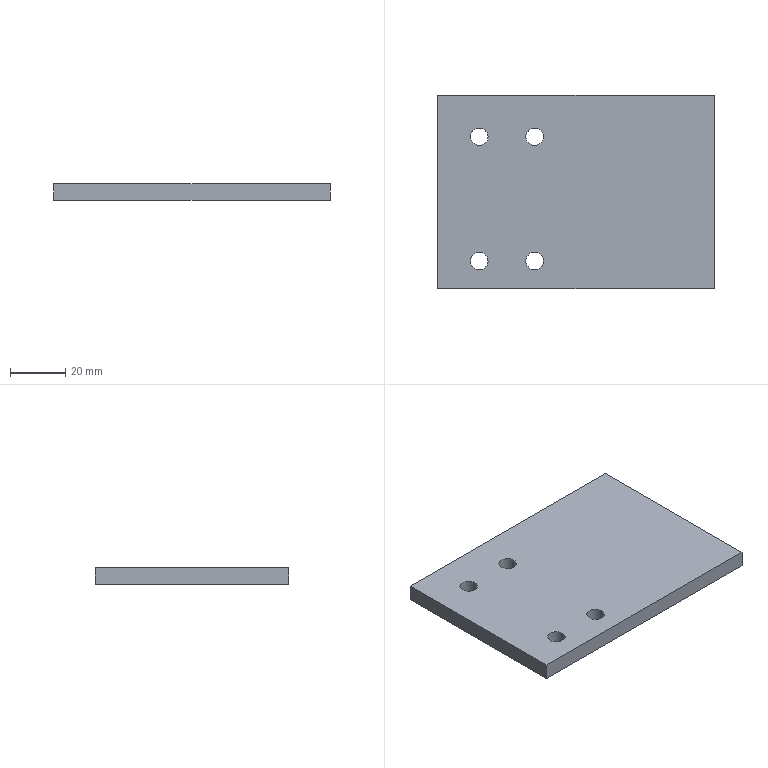Part | SolidWorks | features BaseBody 1 | 1 solid | 14 faces | box 100 x 70 x 6 mm | volume 41252 mm3 | cylinder 8 | plane 6 | commonest cylinder face diameters 6.3 x8
STEP:
#1=CARTESIAN_POINT('',(-18.15,20.,-3.));
#2=VERTEX_POINT('',#1);
#3=CARTESIAN_POINT('',(-11.85,20.,-3.));
#4=VERTEX_POINT('',#3);
#5=CARTESIAN_POINT('',(-15.,20.,-3.));
#6=DIRECTION('',(0.,0.,1.));
#7=DIRECTION('',(1.,0.,0.));
#8=AXIS2_PLACEMENT_3D('',#5,#6,#7);
#9=CIRCLE('',#8,3.15);
#10=EDGE_CURVE('',#2,#4,#9,.T.);
#11=ORIENTED_EDGE('',*,*,#10,.F.);
#12=CARTESIAN_POINT('',(-18.15,20.,3.));
#13=VERTEX_POINT('',#12);
#14=CARTESIAN_POINT('',(-18.15,20.,-15.2));
#15=DIRECTION('',(0.,0.,1.));
#16=VECTOR('',#15,1000.);
#17=LINE('',#14,#16);
#18=EDGE_CURVE('',#2,#13,#17,.T.);
#19=ORIENTED_EDGE('',*,*,#18,.T.);
#20=CARTESIAN_POINT('',(-11.85,20.,3.));
#21=VERTEX_POINT('',#20);
#22=CARTESIAN_POINT('',(-15.,20.,3.));
#23=DIRECTION('',(0.,0.,-1.));
#24=DIRECTION('',(1.,0.,0.));
#25=AXIS2_PLACEMENT_3D('',#22,#23,#24);
#26=CIRCLE('',#25,3.15);
#27=EDGE_CURVE('',#21,#13,#26,.T.);
#28=ORIENTED_EDGE('',*,*,#27,.F.);
#29=CARTESIAN_POINT('',(-11.85,20.,-15.2));
#30=DIRECTION('',(0.,0.,1.));
#31=VECTOR('',#30,1000.);
#32=LINE('',#29,#31);
#33=EDGE_CURVE('',#4,#21,#32,.T.);
#34=ORIENTED_EDGE('',*,*,#33,.F.);
#35=EDGE_LOOP('',(#11,#19,#28,#34));
#36=FACE_OUTER_BOUND('',#35,.T.);
#37=CARTESIAN_POINT('',(-15.,20.,-15.2));
#38=DIRECTION('',(0.,0.,1.));
#39=DIRECTION('',(1.,0.,0.));
#40=AXIS2_PLACEMENT_3D('',#37,#38,#39);
#41=CYLINDRICAL_SURFACE('',#40,3.15);
#42=ADVANCED_FACE('',(#36),#41,.F.);
#43=CARTESIAN_POINT('',(-38.15,20.,-3.));
#44=VERTEX_POINT('',#43);
#45=CARTESIAN_POINT('',(-31.85,20.,-3.));
#46=VERTEX_POINT('',#45);
#47=CARTESIAN_POINT('',(-35.,20.,-3.));
#48=DIRECTION('',(0.,0.,1.));
#49=DIRECTION('',(1.,0.,0.));
#50=AXIS2_PLACEMENT_3D('',#47,#48,#49);
#51=CIRCLE('',#50,3.15);
#52=EDGE_CURVE('',#44,#46,#51,.T.);
#53=ORIENTED_EDGE('',*,*,#52,.F.);
#54=CARTESIAN_POINT('',(-38.15,20.,3.));
#55=VERTEX_POINT('',#54);
#56=CARTESIAN_POINT('',(-38.15,20.,-15.2));
#57=DIRECTION('',(0.,0.,1.));
#58=VECTOR('',#57,1000.);
#59=LINE('',#56,#58);
#60=EDGE_CURVE('',#44,#55,#59,.T.);
#61=ORIENTED_EDGE('',*,*,#60,.T.);
#62=CARTESIAN_POINT('',(-31.85,20.,3.));
#63=VERTEX_POINT('',#62);
#64=CARTESIAN_POINT('',(-35.,20.,3.));
#65=DIRECTION('',(0.,0.,-1.));
#66=DIRECTION('',(1.,0.,0.));
#67=AXIS2_PLACEMENT_3D('',#64,#65,#66);
#68=CIRCLE('',#67,3.15);
#69=EDGE_CURVE('',#63,#55,#68,.T.);
#70=ORIENTED_EDGE('',*,*,#69,.F.);
#71=CARTESIAN_POINT('',(-31.85,20.,-15.2));
#72=DIRECTION('',(0.,0.,1.));
#73=VECTOR('',#72,1000.);
#74=LINE('',#71,#73);
#75=EDGE_CURVE('',#46,#63,#74,.T.);
#76=ORIENTED_EDGE('',*,*,#75,.F.);
#77=EDGE_LOOP('',(#53,#61,#70,#76));
#78=FACE_OUTER_BOUND('',#77,.T.);
#79=CARTESIAN_POINT('',(-35.,20.,-15.2));
#80=DIRECTION('',(0.,0.,1.));
#81=DIRECTION('',(1.,0.,0.));
#82=AXIS2_PLACEMENT_3D('',#79,#80,#81);
#83=CYLINDRICAL_SURFACE('',#82,3.15);
#84=ADVANCED_FACE('',(#78),#83,.F.);
#85=CARTESIAN_POINT('',(-18.15,-25.,-3.));
#86=VERTEX_POINT('',#85);
#87=CARTESIAN_POINT('',(-11.85,-25.,-3.));
#88=VERTEX_POINT('',#87);
#89=CARTESIAN_POINT('',(-15.,-25.,-3.));
#90=DIRECTION('',(0.,0.,1.));
#91=DIRECTION('',(1.,0.,0.));
#92=AXIS2_PLACEMENT_3D('',#89,#90,#91);
#93=CIRCLE('',#92,3.15);
#94=EDGE_CURVE('',#86,#88,#93,.T.);
#95=ORIENTED_EDGE('',*,*,#94,.F.);
#96=CARTESIAN_POINT('',(-18.15,-25.,3.));
#97=VERTEX_POINT('',#96);
#98=CARTESIAN_POINT('',(-18.15,-25.,-15.2));
#99=DIRECTION('',(0.,0.,1.));
#100=VECTOR('',#99,1000.);
#101=LINE('',#98,#100);
#102=EDGE_CURVE('',#86,#97,#101,.T.);
#103=ORIENTED_EDGE('',*,*,#102,.T.);
#104=CARTESIAN_POINT('',(-11.85,-25.,3.));
#105=VERTEX_POINT('',#104);
#106=CARTESIAN_POINT('',(-15.,-25.,3.));
#107=DIRECTION('',(0.,0.,-1.));
#108=DIRECTION('',(1.,0.,0.));
#109=AXIS2_PLACEMENT_3D('',#106,#107,#108);
#110=CIRCLE('',#109,3.15);
#111=EDGE_CURVE('',#105,#97,#110,.T.);
#112=ORIENTED_EDGE('',*,*,#111,.F.);
#113=CARTESIAN_POINT('',(-11.85,-25.,-15.2));
#114=DIRECTION('',(0.,0.,1.));
#115=VECTOR('',#114,1000.);
#116=LINE('',#113,#115);
#117=EDGE_CURVE('',#88,#105,#116,.T.);
#118=ORIENTED_EDGE('',*,*,#117,.F.);
#119=EDGE_LOOP('',(#95,#103,#112,#118));
#120=FACE_OUTER_BOUND('',#119,.T.);
#121=CARTESIAN_POINT('',(-15.,-25.,-15.2));
#122=DIRECTION('',(0.,0.,1.));
#123=DIRECTION('',(1.,0.,0.));
#124=AXIS2_PLACEMENT_3D('',#121,#122,#123);
#125=CYLINDRICAL_SURFACE('',#124,3.15);
#126=ADVANCED_FACE('',(#120),#125,.F.);
#127=CARTESIAN_POINT('',(-38.15,-25.,-3.));
#128=VERTEX_POINT('',#127);
#129=CARTESIAN_POINT('',(-31.85,-25.,-3.));
#130=VERTEX_POINT('',#129);
#131=CARTESIAN_POINT('',(-35.,-25.,-3.));
#132=DIRECTION('',(0.,0.,1.));
#133=DIRECTION('',(1.,0.,0.));
#134=AXIS2_PLACEMENT_3D('',#131,#132,#133);
#135=CIRCLE('',#134,3.15);
#136=EDGE_CURVE('',#128,#130,#135,.T.);
#137=ORIENTED_EDGE('',*,*,#136,.F.);
#138=CARTESIAN_POINT('',(-38.15,-25.,3.));
#139=VERTEX_POINT('',#138);
#140=CARTESIAN_POINT('',(-38.15,-25.,-15.2));
#141=DIRECTION('',(0.,0.,1.));
#142=VECTOR('',#141,1000.);
#143=LINE('',#140,#142);
#144=EDGE_CURVE('',#128,#139,#143,.T.);
#145=ORIENTED_EDGE('',*,*,#144,.T.);
#146=CARTESIAN_POINT('',(-31.85,-25.,3.));
#147=VERTEX_POINT('',#146);
#148=CARTESIAN_POINT('',(-35.,-25.,3.));
#149=DIRECTION('',(0.,0.,-1.));
#150=DIRECTION('',(1.,0.,0.));
#151=AXIS2_PLACEMENT_3D('',#148,#149,#150);
#152=CIRCLE('',#151,3.15);
#153=EDGE_CURVE('',#147,#139,#152,.T.);
#154=ORIENTED_EDGE('',*,*,#153,.F.);
#155=CARTESIAN_POINT('',(-31.85,-25.,-15.2));
#156=DIRECTION('',(0.,0.,1.));
#157=VECTOR('',#156,1000.);
#158=LINE('',#155,#157);
#159=EDGE_CURVE('',#130,#147,#158,.T.);
#160=ORIENTED_EDGE('',*,*,#159,.F.);
#161=EDGE_LOOP('',(#137,#145,#154,#160));
#162=FACE_OUTER_BOUND('',#161,.T.);
#163=CARTESIAN_POINT('',(-35.,-25.,-15.2));
#164=DIRECTION('',(0.,0.,1.));
#165=DIRECTION('',(1.,0.,0.));
#166=AXIS2_PLACEMENT_3D('',#163,#164,#165);
#167=CYLINDRICAL_SURFACE('',#166,3.15);
#168=ADVANCED_FACE('',(#162),#167,.F.);
#169=ORIENTED_EDGE('',*,*,#27,.T.);
#170=CARTESIAN_POINT('',(-15.,20.,3.));
#171=DIRECTION('',(0.,0.,-1.));
#172=DIRECTION('',(1.,0.,0.));
#173=AXIS2_PLACEMENT_3D('',#170,#171,#172);
#174=CIRCLE('',#173,3.15);
#175=EDGE_CURVE('',#13,#21,#174,.T.);
#176=ORIENTED_EDGE('',*,*,#175,.T.);
#177=EDGE_LOOP('',(#169,#176));
#178=FACE_BOUND('',#177,.T.);
#179=ORIENTED_EDGE('',*,*,#69,.T.);
#180=CARTESIAN_POINT('',(-35.,20.,3.));
#181=DIRECTION('',(0.,0.,-1.));
#182=DIRECTION('',(1.,0.,0.));
#183=AXIS2_PLACEMENT_3D('',#180,#181,#182);
#184=CIRCLE('',#183,3.15);
#185=EDGE_CURVE('',#55,#63,#184,.T.);
#186=ORIENTED_EDGE('',*,*,#185,.T.);
#187=EDGE_LOOP('',(#179,#186));
#188=FACE_BOUND('',#187,.T.);
#189=ORIENTED_EDGE('',*,*,#111,.T.);
#190=CARTESIAN_POINT('',(-15.,-25.,3.));
#191=DIRECTION('',(0.,0.,-1.));
#192=DIRECTION('',(1.,0.,0.));
#193=AXIS2_PLACEMENT_3D('',#190,#191,#192);
#194=CIRCLE('',#193,3.15);
#195=EDGE_CURVE('',#97,#105,#194,.T.);
#196=ORIENTED_EDGE('',*,*,#195,.T.);
#197=EDGE_LOOP('',(#189,#196));
#198=FACE_BOUND('',#197,.T.);
#199=ORIENTED_EDGE('',*,*,#153,.T.);
#200=CARTESIAN_POINT('',(-35.,-25.,3.));
#201=DIRECTION('',(0.,0.,-1.));
#202=DIRECTION('',(1.,0.,0.));
#203=AXIS2_PLACEMENT_3D('',#200,#201,#202);
#204=CIRCLE('',#203,3.15);
#205=EDGE_CURVE('',#139,#147,#204,.T.);
#206=ORIENTED_EDGE('',*,*,#205,.T.);
#207=EDGE_LOOP('',(#199,#206));
#208=FACE_BOUND('',#207,.T.);
#209=CARTESIAN_POINT('',(50.,-35.,3.));
#210=VERTEX_POINT('',#209);
#211=CARTESIAN_POINT('',(50.,35.,3.));
#212=VERTEX_POINT('',#211);
#213=CARTESIAN_POINT('',(50.,-35.,3.));
#214=DIRECTION('',(0.,1.,0.));
#215=VECTOR('',#214,1000.);
#216=LINE('',#213,#215);
#217=EDGE_CURVE('',#210,#212,#216,.T.);
#218=ORIENTED_EDGE('',*,*,#217,.T.);
#219=CARTESIAN_POINT('',(-50.,35.,3.));
#220=VERTEX_POINT('',#219);
#221=CARTESIAN_POINT('',(-50.,35.,3.));
#222=DIRECTION('',(-1.,0.,0.));
#223=VECTOR('',#222,1000.);
#224=LINE('',#221,#223);
#225=EDGE_CURVE('',#212,#220,#224,.T.);
#226=ORIENTED_EDGE('',*,*,#225,.T.);
#227=CARTESIAN_POINT('',(-50.,-35.,3.));
#228=VERTEX_POINT('',#227);
#229=CARTESIAN_POINT('',(-50.,-35.,3.));
#230=DIRECTION('',(0.,-1.,0.));
#231=VECTOR('',#230,1000.);
#232=LINE('',#229,#231);
#233=EDGE_CURVE('',#220,#228,#232,.T.);
#234=ORIENTED_EDGE('',*,*,#233,.T.);
#235=CARTESIAN_POINT('',(-50.,-35.,3.));
#236=DIRECTION('',(1.,0.,0.));
#237=VECTOR('',#236,1000.);
#238=LINE('',#235,#237);
#239=EDGE_CURVE('',#228,#210,#238,.T.);
#240=ORIENTED_EDGE('',*,*,#239,.T.);
#241=EDGE_LOOP('',(#218,#226,#234,#240));
#242=FACE_OUTER_BOUND('',#241,.T.);
#243=CARTESIAN_POINT('',(-50.,-35.,3.));
#244=DIRECTION('',(0.,0.,1.));
#245=DIRECTION('',(1.,0.,0.));
#246=AXIS2_PLACEMENT_3D('',#243,#244,#245);
#247=PLANE('',#246);
#248=ADVANCED_FACE('',(#178,#188,#198,#208,#242),#247,.T.);
#249=ORIENTED_EDGE('',*,*,#18,.F.);
#250=CARTESIAN_POINT('',(-15.,20.,-3.));
#251=DIRECTION('',(0.,0.,1.));
#252=DIRECTION('',(1.,0.,0.));
#253=AXIS2_PLACEMENT_3D('',#250,#251,#252);
#254=CIRCLE('',#253,3.15);
#255=EDGE_CURVE('',#4,#2,#254,.T.);
#256=ORIENTED_EDGE('',*,*,#255,.F.);
#257=ORIENTED_EDGE('',*,*,#33,.T.);
#258=ORIENTED_EDGE('',*,*,#175,.F.);
#259=EDGE_LOOP('',(#249,#256,#257,#258));
#260=FACE_OUTER_BOUND('',#259,.T.);
#261=CARTESIAN_POINT('',(-15.,20.,-15.2));
#262=DIRECTION('',(0.,0.,1.));
#263=DIRECTION('',(1.,0.,0.));
#264=AXIS2_PLACEMENT_3D('',#261,#262,#263);
#265=CYLINDRICAL_SURFACE('',#264,3.15);
#266=ADVANCED_FACE('',(#260),#265,.F.);
#267=ORIENTED_EDGE('',*,*,#60,.F.);
#268=CARTESIAN_POINT('',(-35.,20.,-3.));
#269=DIRECTION('',(0.,0.,1.));
#270=DIRECTION('',(1.,0.,0.));
#271=AXIS2_PLACEMENT_3D('',#268,#269,#270);
#272=CIRCLE('',#271,3.15);
#273=EDGE_CURVE('',#46,#44,#272,.T.);
#274=ORIENTED_EDGE('',*,*,#273,.F.);
#275=ORIENTED_EDGE('',*,*,#75,.T.);
#276=ORIENTED_EDGE('',*,*,#185,.F.);
#277=EDGE_LOOP('',(#267,#274,#275,#276));
#278=FACE_OUTER_BOUND('',#277,.T.);
#279=CARTESIAN_POINT('',(-35.,20.,-15.2));
#280=DIRECTION('',(0.,0.,1.));
#281=DIRECTION('',(1.,0.,0.));
#282=AXIS2_PLACEMENT_3D('',#279,#280,#281);
#283=CYLINDRICAL_SURFACE('',#282,3.15);
#284=ADVANCED_FACE('',(#278),#283,.F.);
#285=ORIENTED_EDGE('',*,*,#102,.F.);
#286=CARTESIAN_POINT('',(-15.,-25.,-3.));
#287=DIRECTION('',(0.,0.,1.));
#288=DIRECTION('',(1.,0.,0.));
#289=AXIS2_PLACEMENT_3D('',#286,#287,#288);
#290=CIRCLE('',#289,3.15);
#291=EDGE_CURVE('',#88,#86,#290,.T.);
#292=ORIENTED_EDGE('',*,*,#291,.F.);
#293=ORIENTED_EDGE('',*,*,#117,.T.);
#294=ORIENTED_EDGE('',*,*,#195,.F.);
#295=EDGE_LOOP('',(#285,#292,#293,#294));
#296=FACE_OUTER_BOUND('',#295,.T.);
#297=CARTESIAN_POINT('',(-15.,-25.,-15.2));
#298=DIRECTION('',(0.,0.,1.));
#299=DIRECTION('',(1.,0.,0.));
#300=AXIS2_PLACEMENT_3D('',#297,#298,#299);
#301=CYLINDRICAL_SURFACE('',#300,3.15);
#302=ADVANCED_FACE('',(#296),#301,.F.);
#303=ORIENTED_EDGE('',*,*,#144,.F.);
#304=CARTESIAN_POINT('',(-35.,-25.,-3.));
#305=DIRECTION('',(0.,0.,1.));
#306=DIRECTION('',(1.,0.,0.));
#307=AXIS2_PLACEMENT_3D('',#304,#305,#306);
#308=CIRCLE('',#307,3.15);
#309=EDGE_CURVE('',#130,#128,#308,.T.);
#310=ORIENTED_EDGE('',*,*,#309,.F.);
#311=ORIENTED_EDGE('',*,*,#159,.T.);
#312=ORIENTED_EDGE('',*,*,#205,.F.);
#313=EDGE_LOOP('',(#303,#310,#311,#312));
#314=FACE_OUTER_BOUND('',#313,.T.);
#315=CARTESIAN_POINT('',(-35.,-25.,-15.2));
#316=DIRECTION('',(0.,0.,1.));
#317=DIRECTION('',(1.,0.,0.));
#318=AXIS2_PLACEMENT_3D('',#315,#316,#317);
#319=CYLINDRICAL_SURFACE('',#318,3.15);
#320=ADVANCED_FACE('',(#314),#319,.F.);
#321=ORIENTED_EDGE('',*,*,#225,.F.);
#322=CARTESIAN_POINT('',(50.,35.,-3.));
#323=VERTEX_POINT('',#322);
#324=CARTESIAN_POINT('',(50.,35.,-3.));
#325=DIRECTION('',(0.,0.,-1.));
#326=VECTOR('',#325,1000.);
#327=LINE('',#324,#326);
#328=EDGE_CURVE('',#212,#323,#327,.T.);
#329=ORIENTED_EDGE('',*,*,#328,.T.);
#330=CARTESIAN_POINT('',(-50.,35.,-3.));
#331=VERTEX_POINT('',#330);
#332=CARTESIAN_POINT('',(-50.,35.,-3.));
#333=DIRECTION('',(-1.,0.,0.));
#334=VECTOR('',#333,1000.);
#335=LINE('',#332,#334);
#336=EDGE_CURVE('',#323,#331,#335,.T.);
#337=ORIENTED_EDGE('',*,*,#336,.T.);
#338=CARTESIAN_POINT('',(-50.,35.,-3.));
#339=DIRECTION('',(0.,0.,1.));
#340=VECTOR('',#339,1000.);
#341=LINE('',#338,#340);
#342=EDGE_CURVE('',#331,#220,#341,.T.);
#343=ORIENTED_EDGE('',*,*,#342,.T.);
#344=EDGE_LOOP('',(#321,#329,#337,#343));
#345=FACE_OUTER_BOUND('',#344,.T.);
#346=CARTESIAN_POINT('',(-50.,35.,-3.));
#347=DIRECTION('',(0.,1.,0.));
#348=DIRECTION('',(0.,0.,1.));
#349=AXIS2_PLACEMENT_3D('',#346,#347,#348);
#350=PLANE('',#349);
#351=ADVANCED_FACE('',(#345),#350,.T.);
#352=ORIENTED_EDGE('',*,*,#328,.F.);
#353=ORIENTED_EDGE('',*,*,#217,.F.);
#354=CARTESIAN_POINT('',(50.,-35.,-3.));
#355=VERTEX_POINT('',#354);
#356=CARTESIAN_POINT('',(50.,-35.,-3.));
#357=DIRECTION('',(0.,0.,-1.));
#358=VECTOR('',#357,1000.);
#359=LINE('',#356,#358);
#360=EDGE_CURVE('',#210,#355,#359,.T.);
#361=ORIENTED_EDGE('',*,*,#360,.T.);
#362=CARTESIAN_POINT('',(50.,-35.,-3.));
#363=DIRECTION('',(0.,1.,0.));
#364=VECTOR('',#363,1000.);
#365=LINE('',#362,#364);
#366=EDGE_CURVE('',#355,#323,#365,.T.);
#367=ORIENTED_EDGE('',*,*,#366,.T.);
#368=EDGE_LOOP('',(#352,#353,#361,#367));
#369=FACE_OUTER_BOUND('',#368,.T.);
#370=CARTESIAN_POINT('',(50.,-35.,-3.));
#371=DIRECTION('',(1.,0.,0.));
#372=DIRECTION('',(0.,0.,-1.));
#373=AXIS2_PLACEMENT_3D('',#370,#371,#372);
#374=PLANE('',#373);
#375=ADVANCED_FACE('',(#369),#374,.T.);
#376=ORIENTED_EDGE('',*,*,#239,.F.);
#377=CARTESIAN_POINT('',(-50.,-35.,-3.));
#378=VERTEX_POINT('',#377);
#379=CARTESIAN_POINT('',(-50.,-35.,-3.));
#380=DIRECTION('',(0.,0.,1.));
#381=VECTOR('',#380,1000.);
#382=LINE('',#379,#381);
#383=EDGE_CURVE('',#378,#228,#382,.T.);
#384=ORIENTED_EDGE('',*,*,#383,.F.);
#385=CARTESIAN_POINT('',(-50.,-35.,-3.));
#386=DIRECTION('',(-1.,0.,0.));
#387=VECTOR('',#386,1000.);
#388=LINE('',#385,#387);
#389=EDGE_CURVE('',#355,#378,#388,.T.);
#390=ORIENTED_EDGE('',*,*,#389,.F.);
#391=ORIENTED_EDGE('',*,*,#360,.F.);
#392=EDGE_LOOP('',(#376,#384,#390,#391));
#393=FACE_OUTER_BOUND('',#392,.T.);
#394=CARTESIAN_POINT('',(-50.,-35.,-3.));
#395=DIRECTION('',(0.,1.,0.));
#396=DIRECTION('',(0.,0.,1.));
#397=AXIS2_PLACEMENT_3D('',#394,#395,#396);
#398=PLANE('',#397);
#399=ADVANCED_FACE('',(#393),#398,.F.);
#400=ORIENTED_EDGE('',*,*,#342,.F.);
#401=CARTESIAN_POINT('',(-50.,-35.,-3.));
#402=DIRECTION('',(0.,1.,0.));
#403=VECTOR('',#402,1000.);
#404=LINE('',#401,#403);
#405=EDGE_CURVE('',#378,#331,#404,.T.);
#406=ORIENTED_EDGE('',*,*,#405,.F.);
#407=ORIENTED_EDGE('',*,*,#383,.T.);
#408=ORIENTED_EDGE('',*,*,#233,.F.);
#409=EDGE_LOOP('',(#400,#406,#407,#408));
#410=FACE_OUTER_BOUND('',#409,.T.);
#411=CARTESIAN_POINT('',(-50.,-35.,-3.));
#412=DIRECTION('',(1.,0.,0.));
#413=DIRECTION('',(0.,0.,-1.));
#414=AXIS2_PLACEMENT_3D('',#411,#412,#413);
#415=PLANE('',#414);
#416=ADVANCED_FACE('',(#410),#415,.F.);
#417=ORIENTED_EDGE('',*,*,#255,.T.);
#418=ORIENTED_EDGE('',*,*,#10,.T.);
#419=EDGE_LOOP('',(#417,#418));
#420=FACE_BOUND('',#419,.T.);
#421=ORIENTED_EDGE('',*,*,#273,.T.);
#422=ORIENTED_EDGE('',*,*,#52,.T.);
#423=EDGE_LOOP('',(#421,#422));
#424=FACE_BOUND('',#423,.T.);
#425=ORIENTED_EDGE('',*,*,#291,.T.);
#426=ORIENTED_EDGE('',*,*,#94,.T.);
#427=EDGE_LOOP('',(#425,#426));
#428=FACE_BOUND('',#427,.T.);
#429=ORIENTED_EDGE('',*,*,#309,.T.);
#430=ORIENTED_EDGE('',*,*,#136,.T.);
#431=EDGE_LOOP('',(#429,#430));
#432=FACE_BOUND('',#431,.T.);
#433=ORIENTED_EDGE('',*,*,#366,.F.);
#434=ORIENTED_EDGE('',*,*,#389,.T.);
#435=ORIENTED_EDGE('',*,*,#405,.T.);
#436=ORIENTED_EDGE('',*,*,#336,.F.);
#437=EDGE_LOOP('',(#433,#434,#435,#436));
#438=FACE_OUTER_BOUND('',#437,.T.);
#439=CARTESIAN_POINT('',(-50.,-35.,-3.));
#440=DIRECTION('',(0.,0.,1.));
#441=DIRECTION('',(1.,0.,0.));
#442=AXIS2_PLACEMENT_3D('',#439,#440,#441);
#443=PLANE('',#442);
#444=ADVANCED_FACE('',(#420,#424,#428,#432,#438),#443,.F.);
#445=CLOSED_SHELL('',(#42,#84,#126,#168,#248,#266,#284,#302,#320,#351,#375,#399,#416,#444));
#446=MANIFOLD_SOLID_BREP('',#445);
#447=CARTESIAN_POINT('',(0.,0.,0.));
#448=DIRECTION('',(0.,0.,1.));
#449=DIRECTION('',(1.,0.,0.));
#450=AXIS2_PLACEMENT_3D('',#447,#448,#449);
#451=(LENGTH_UNIT()NAMED_UNIT(*)SI_UNIT(.MILLI.,.METRE.));
#452=UNCERTAINTY_MEASURE_WITH_UNIT(LENGTH_MEASURE(0.00001),#451,'','');
#453=(NAMED_UNIT(*)PLANE_ANGLE_UNIT()SI_UNIT($,.RADIAN.));
#454=(NAMED_UNIT(*)SI_UNIT($,.STERADIAN.)SOLID_ANGLE_UNIT());
#455=(GEOMETRIC_REPRESENTATION_CONTEXT(3)GLOBAL_UNCERTAINTY_ASSIGNED_CONTEXT((#452))GLOBAL_UNIT_ASSIGNED_CONTEXT((#451,#453,#454))REPRESENTATION_CONTEXT('',''));
#456=ADVANCED_BREP_SHAPE_REPRESENTATION('',(#446,#450),#455);